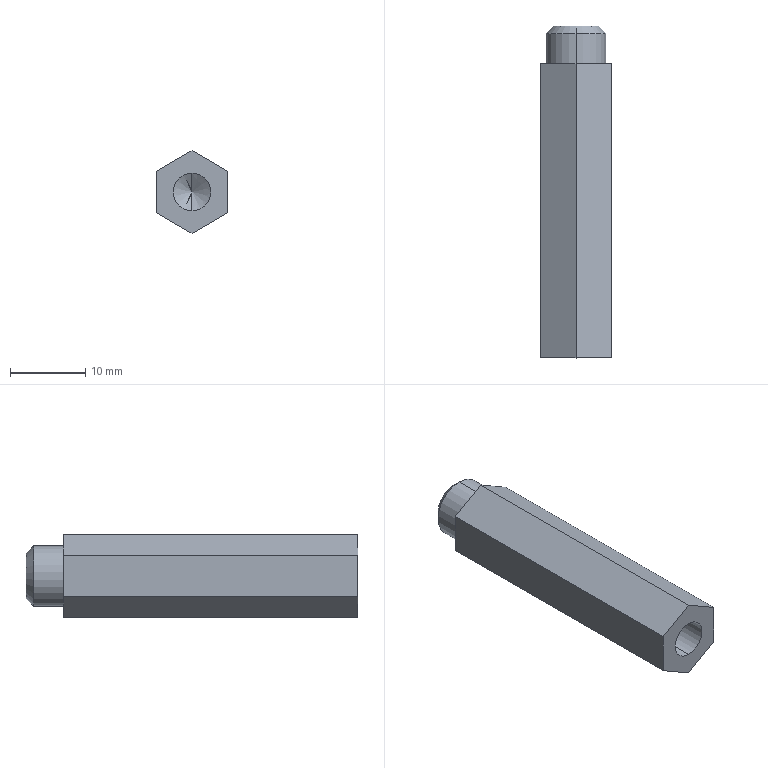Part | SolidWorks | features 3DProfileFeature 1, Chamfer 1, Extrusion 1, HoleWzd 1, ICE 1 | 1 solid | 17 faces | box 9.526 x 44 x 11 mm | volume 3138 mm3 | plane 9 | cylinder 4 | cone 4 | commonest cylinder face diameters 5 x2 8 x2
STEP:
#1=CARTESIAN_POINT('',(-0.000004548,-11.5,2.5));
#2=VERTEX_POINT('',#1);
#3=CARTESIAN_POINT('',(-0.000004548,-11.5,-2.5));
#4=VERTEX_POINT('',#3);
#5=CARTESIAN_POINT('',(-0.000004548,-11.5,0.00002582));
#6=DIRECTION('',(0.,-1.,0.));
#7=DIRECTION('',(0.,0.,-1.));
#8=AXIS2_PLACEMENT_3D('',#5,#6,#7);
#9=CIRCLE('',#8,2.5);
#10=EDGE_CURVE('',#2,#4,#9,.T.);
#11=ORIENTED_EDGE('',*,*,#10,.F.);
#12=CARTESIAN_POINT('',(-0.000004548,-19.5,2.5));
#13=VERTEX_POINT('',#12);
#14=CARTESIAN_POINT('',(-0.000004548,-19.5,2.5));
#15=DIRECTION('',(0.,-1.,0.));
#16=VECTOR('',#15,1000.);
#17=LINE('',#14,#16);
#18=EDGE_CURVE('',#2,#13,#17,.T.);
#19=ORIENTED_EDGE('',*,*,#18,.T.);
#20=CARTESIAN_POINT('',(-0.000004548,-19.5,-2.5));
#21=VERTEX_POINT('',#20);
#22=CARTESIAN_POINT('',(-0.000004548,-19.5,0.00002582));
#23=DIRECTION('',(0.,-1.,0.));
#24=DIRECTION('',(0.,0.,-1.));
#25=AXIS2_PLACEMENT_3D('',#22,#23,#24);
#26=CIRCLE('',#25,2.5);
#27=EDGE_CURVE('',#13,#21,#26,.T.);
#28=ORIENTED_EDGE('',*,*,#27,.T.);
#29=CARTESIAN_POINT('',(-0.000004548,-19.5,-2.5));
#30=DIRECTION('',(0.,-1.,0.));
#31=VECTOR('',#30,1000.);
#32=LINE('',#29,#31);
#33=EDGE_CURVE('',#4,#21,#32,.T.);
#34=ORIENTED_EDGE('',*,*,#33,.F.);
#35=EDGE_LOOP('',(#11,#19,#28,#34));
#36=FACE_OUTER_BOUND('',#35,.T.);
#37=CARTESIAN_POINT('',(-0.000004548,-19.5,0.00002582));
#38=DIRECTION('',(0.,-1.,0.));
#39=DIRECTION('',(0.,0.,-1.));
#40=AXIS2_PLACEMENT_3D('',#37,#38,#39);
#41=CYLINDRICAL_SURFACE('',#40,2.5);
#42=ADVANCED_FACE('',(#36),#41,.F.);
#43=CARTESIAN_POINT('',(-0.000004548,-9.998,0.00002582));
#44=VERTEX_POINT('',#43);
#45=CARTESIAN_POINT('',(-0.000004548,-11.5,-2.5));
#46=DIRECTION('',(0.,-0.515,-0.8572));
#47=VECTOR('',#46,1000.);
#48=LINE('',#45,#47);
#49=EDGE_CURVE('',#44,#4,#48,.T.);
#50=ORIENTED_EDGE('',*,*,#49,.F.);
#51=CARTESIAN_POINT('',(-0.000004548,-11.5,2.5));
#52=DIRECTION('',(0.,-0.515,0.8572));
#53=VECTOR('',#52,1000.);
#54=LINE('',#51,#53);
#55=EDGE_CURVE('',#44,#2,#54,.T.);
#56=ORIENTED_EDGE('',*,*,#55,.T.);
#57=ORIENTED_EDGE('',*,*,#10,.T.);
#58=EDGE_LOOP('',(#50,#56,#57));
#59=FACE_OUTER_BOUND('',#58,.T.);
#60=CARTESIAN_POINT('',(-0.000004548,-11.5,0.00002582));
#61=DIRECTION('',(0.,-1.,0.));
#62=DIRECTION('',(0.,0.,-1.));
#63=AXIS2_PLACEMENT_3D('',#60,#61,#62);
#64=CONICAL_SURFACE('',#63,2.5,1.03);
#65=ADVANCED_FACE('',(#59),#64,.F.);
#66=CARTESIAN_POINT('',(0.,24.5,3.));
#67=VERTEX_POINT('',#66);
#68=CARTESIAN_POINT('',(0.,24.5,-3.));
#69=VERTEX_POINT('',#68);
#70=CARTESIAN_POINT('',(0.,24.5,0.));
#71=DIRECTION('',(0.,1.,0.));
#72=DIRECTION('',(0.,0.,1.));
#73=AXIS2_PLACEMENT_3D('',#70,#71,#72);
#74=CIRCLE('',#73,3.);
#75=EDGE_CURVE('',#67,#69,#74,.T.);
#76=ORIENTED_EDGE('',*,*,#75,.F.);
#77=CARTESIAN_POINT('',(0.,23.5,4.));
#78=VERTEX_POINT('',#77);
#79=CARTESIAN_POINT('',(0.,24.5,3.));
#80=DIRECTION('',(0.,-0.7071,0.7071));
#81=VECTOR('',#80,1000.);
#82=LINE('',#79,#81);
#83=EDGE_CURVE('',#67,#78,#82,.T.);
#84=ORIENTED_EDGE('',*,*,#83,.T.);
#85=CARTESIAN_POINT('',(0.,23.5,-4.));
#86=VERTEX_POINT('',#85);
#87=CARTESIAN_POINT('',(0.,23.5,0.));
#88=DIRECTION('',(0.,-1.,0.));
#89=DIRECTION('',(0.,0.,1.));
#90=AXIS2_PLACEMENT_3D('',#87,#88,#89);
#91=CIRCLE('',#90,4.);
#92=EDGE_CURVE('',#86,#78,#91,.T.);
#93=ORIENTED_EDGE('',*,*,#92,.F.);
#94=CARTESIAN_POINT('',(0.,24.5,-3.));
#95=DIRECTION('',(0.,-0.7071,-0.7071));
#96=VECTOR('',#95,1000.);
#97=LINE('',#94,#96);
#98=EDGE_CURVE('',#69,#86,#97,.T.);
#99=ORIENTED_EDGE('',*,*,#98,.F.);
#100=EDGE_LOOP('',(#76,#84,#93,#99));
#101=FACE_OUTER_BOUND('',#100,.T.);
#102=CARTESIAN_POINT('',(0.,24.5,0.));
#103=DIRECTION('',(0.,-1.,0.));
#104=DIRECTION('',(0.,0.,-1.));
#105=AXIS2_PLACEMENT_3D('',#102,#103,#104);
#106=CONICAL_SURFACE('',#105,3.,0.7854);
#107=ADVANCED_FACE('',(#101),#106,.T.);
#108=ORIENTED_EDGE('',*,*,#92,.T.);
#109=CARTESIAN_POINT('',(0.,19.5,4.));
#110=VERTEX_POINT('',#109);
#111=CARTESIAN_POINT('',(0.,24.5,4.));
#112=DIRECTION('',(0.,-1.,0.));
#113=VECTOR('',#112,1000.);
#114=LINE('',#111,#113);
#115=EDGE_CURVE('',#78,#110,#114,.T.);
#116=ORIENTED_EDGE('',*,*,#115,.T.);
#117=CARTESIAN_POINT('',(0.,19.5,-4.));
#118=VERTEX_POINT('',#117);
#119=CARTESIAN_POINT('',(0.,19.5,0.));
#120=DIRECTION('',(0.,1.,0.));
#121=DIRECTION('',(0.,0.,1.));
#122=AXIS2_PLACEMENT_3D('',#119,#120,#121);
#123=CIRCLE('',#122,4.);
#124=EDGE_CURVE('',#110,#118,#123,.T.);
#125=ORIENTED_EDGE('',*,*,#124,.T.);
#126=CARTESIAN_POINT('',(0.,24.5,-4.));
#127=DIRECTION('',(0.,-1.,0.));
#128=VECTOR('',#127,1000.);
#129=LINE('',#126,#128);
#130=EDGE_CURVE('',#86,#118,#129,.T.);
#131=ORIENTED_EDGE('',*,*,#130,.F.);
#132=EDGE_LOOP('',(#108,#116,#125,#131));
#133=FACE_OUTER_BOUND('',#132,.T.);
#134=CARTESIAN_POINT('',(0.,24.5,0.));
#135=DIRECTION('',(0.,-1.,0.));
#136=DIRECTION('',(0.,0.,-1.));
#137=AXIS2_PLACEMENT_3D('',#134,#135,#136);
#138=CYLINDRICAL_SURFACE('',#137,4.);
#139=ADVANCED_FACE('',(#133),#138,.T.);
#140=CARTESIAN_POINT('',(4.763,19.5,-2.75));
#141=VERTEX_POINT('',#140);
#142=CARTESIAN_POINT('',(0.,19.5,-5.5));
#143=VERTEX_POINT('',#142);
#144=CARTESIAN_POINT('',(4.763,19.5,-2.75));
#145=DIRECTION('',(-0.866,0.,-0.5));
#146=VECTOR('',#145,1000.);
#147=LINE('',#144,#146);
#148=EDGE_CURVE('',#141,#143,#147,.T.);
#149=ORIENTED_EDGE('',*,*,#148,.T.);
#150=CARTESIAN_POINT('',(-4.763,19.5,-2.75));
#151=VERTEX_POINT('',#150);
#152=CARTESIAN_POINT('',(0.,19.5,-5.5));
#153=DIRECTION('',(-0.866,0.,0.5));
#154=VECTOR('',#153,1000.);
#155=LINE('',#152,#154);
#156=EDGE_CURVE('',#143,#151,#155,.T.);
#157=ORIENTED_EDGE('',*,*,#156,.T.);
#158=CARTESIAN_POINT('',(-4.763,19.5,2.75));
#159=VERTEX_POINT('',#158);
#160=CARTESIAN_POINT('',(-4.763,19.5,-2.75));
#161=DIRECTION('',(0.,0.,1.));
#162=VECTOR('',#161,1000.);
#163=LINE('',#160,#162);
#164=EDGE_CURVE('',#151,#159,#163,.T.);
#165=ORIENTED_EDGE('',*,*,#164,.T.);
#166=CARTESIAN_POINT('',(0.,19.5,5.5));
#167=VERTEX_POINT('',#166);
#168=CARTESIAN_POINT('',(-4.763,19.5,2.75));
#169=DIRECTION('',(0.866,0.,0.5));
#170=VECTOR('',#169,1000.);
#171=LINE('',#168,#170);
#172=EDGE_CURVE('',#159,#167,#171,.T.);
#173=ORIENTED_EDGE('',*,*,#172,.T.);
#174=CARTESIAN_POINT('',(4.763,19.5,2.75));
#175=VERTEX_POINT('',#174);
#176=CARTESIAN_POINT('',(0.,19.5,5.5));
#177=DIRECTION('',(0.866,0.,-0.5));
#178=VECTOR('',#177,1000.);
#179=LINE('',#176,#178);
#180=EDGE_CURVE('',#167,#175,#179,.T.);
#181=ORIENTED_EDGE('',*,*,#180,.T.);
#182=CARTESIAN_POINT('',(4.763,19.5,2.75));
#183=DIRECTION('',(0.,0.,-1.));
#184=VECTOR('',#183,1000.);
#185=LINE('',#182,#184);
#186=EDGE_CURVE('',#175,#141,#185,.T.);
#187=ORIENTED_EDGE('',*,*,#186,.T.);
#188=EDGE_LOOP('',(#149,#157,#165,#173,#181,#187));
#189=FACE_OUTER_BOUND('',#188,.T.);
#190=CARTESIAN_POINT('',(0.,19.5,0.));
#191=DIRECTION('',(0.,1.,0.));
#192=DIRECTION('',(0.,0.,1.));
#193=AXIS2_PLACEMENT_3D('',#190,#191,#192);
#194=CIRCLE('',#193,4.);
#195=EDGE_CURVE('',#118,#110,#194,.T.);
#196=ORIENTED_EDGE('',*,*,#195,.F.);
#197=ORIENTED_EDGE('',*,*,#124,.F.);
#198=EDGE_LOOP('',(#196,#197));
#199=FACE_BOUND('',#198,.T.);
#200=CARTESIAN_POINT('',(0.,19.5,0.));
#201=DIRECTION('',(0.,1.,0.));
#202=DIRECTION('',(0.,0.,1.));
#203=AXIS2_PLACEMENT_3D('',#200,#201,#202);
#204=PLANE('',#203);
#205=ADVANCED_FACE('',(#189,#199),#204,.T.);
#206=CARTESIAN_POINT('',(4.763,-19.5,-2.75));
#207=VERTEX_POINT('',#206);
#208=CARTESIAN_POINT('',(0.,-19.5,-5.5));
#209=VERTEX_POINT('',#208);
#210=CARTESIAN_POINT('',(4.763,-19.5,-2.75));
#211=DIRECTION('',(-0.866,0.,-0.5));
#212=VECTOR('',#211,1000.);
#213=LINE('',#210,#212);
#214=EDGE_CURVE('',#207,#209,#213,.T.);
#215=ORIENTED_EDGE('',*,*,#214,.T.);
#216=CARTESIAN_POINT('',(0.,19.5,-5.5));
#217=DIRECTION('',(0.,-1.,0.));
#218=VECTOR('',#217,1000.);
#219=LINE('',#216,#218);
#220=EDGE_CURVE('',#143,#209,#219,.T.);
#221=ORIENTED_EDGE('',*,*,#220,.F.);
#222=ORIENTED_EDGE('',*,*,#148,.F.);
#223=CARTESIAN_POINT('',(4.763,19.5,-2.75));
#224=DIRECTION('',(0.,-1.,0.));
#225=VECTOR('',#224,1000.);
#226=LINE('',#223,#225);
#227=EDGE_CURVE('',#141,#207,#226,.T.);
#228=ORIENTED_EDGE('',*,*,#227,.T.);
#229=EDGE_LOOP('',(#215,#221,#222,#228));
#230=FACE_OUTER_BOUND('',#229,.T.);
#231=CARTESIAN_POINT('',(4.763,19.5,-2.75));
#232=DIRECTION('',(-0.5,0.,0.866));
#233=DIRECTION('',(0.866,0.,0.5));
#234=AXIS2_PLACEMENT_3D('',#231,#232,#233);
#235=PLANE('',#234);
#236=ADVANCED_FACE('',(#230),#235,.F.);
#237=CARTESIAN_POINT('',(-4.763,-19.5,-2.75));
#238=VERTEX_POINT('',#237);
#239=CARTESIAN_POINT('',(0.,-19.5,-5.5));
#240=DIRECTION('',(-0.866,0.,0.5));
#241=VECTOR('',#240,1000.);
#242=LINE('',#239,#241);
#243=EDGE_CURVE('',#209,#238,#242,.T.);
#244=ORIENTED_EDGE('',*,*,#243,.T.);
#245=CARTESIAN_POINT('',(-4.763,19.5,-2.75));
#246=DIRECTION('',(0.,-1.,0.));
#247=VECTOR('',#246,1000.);
#248=LINE('',#245,#247);
#249=EDGE_CURVE('',#151,#238,#248,.T.);
#250=ORIENTED_EDGE('',*,*,#249,.F.);
#251=ORIENTED_EDGE('',*,*,#156,.F.);
#252=ORIENTED_EDGE('',*,*,#220,.T.);
#253=EDGE_LOOP('',(#244,#250,#251,#252));
#254=FACE_OUTER_BOUND('',#253,.T.);
#255=CARTESIAN_POINT('',(0.,19.5,-5.5));
#256=DIRECTION('',(0.5,0.,0.866));
#257=DIRECTION('',(0.866,0.,-0.5));
#258=AXIS2_PLACEMENT_3D('',#255,#256,#257);
#259=PLANE('',#258);
#260=ADVANCED_FACE('',(#254),#259,.F.);
#261=CARTESIAN_POINT('',(-4.763,-19.5,2.75));
#262=VERTEX_POINT('',#261);
#263=CARTESIAN_POINT('',(-4.763,-19.5,-2.75));
#264=DIRECTION('',(0.,0.,1.));
#265=VECTOR('',#264,1000.);
#266=LINE('',#263,#265);
#267=EDGE_CURVE('',#238,#262,#266,.T.);
#268=ORIENTED_EDGE('',*,*,#267,.T.);
#269=CARTESIAN_POINT('',(-4.763,19.5,2.75));
#270=DIRECTION('',(0.,-1.,0.));
#271=VECTOR('',#270,1000.);
#272=LINE('',#269,#271);
#273=EDGE_CURVE('',#159,#262,#272,.T.);
#274=ORIENTED_EDGE('',*,*,#273,.F.);
#275=ORIENTED_EDGE('',*,*,#164,.F.);
#276=ORIENTED_EDGE('',*,*,#249,.T.);
#277=EDGE_LOOP('',(#268,#274,#275,#276));
#278=FACE_OUTER_BOUND('',#277,.T.);
#279=CARTESIAN_POINT('',(-4.763,19.5,-2.75));
#280=DIRECTION('',(1.,0.,0.));
#281=DIRECTION('',(0.,0.,-1.));
#282=AXIS2_PLACEMENT_3D('',#279,#280,#281);
#283=PLANE('',#282);
#284=ADVANCED_FACE('',(#278),#283,.F.);
#285=CARTESIAN_POINT('',(0.,-19.5,5.5));
#286=VERTEX_POINT('',#285);
#287=CARTESIAN_POINT('',(-4.763,-19.5,2.75));
#288=DIRECTION('',(0.866,0.,0.5));
#289=VECTOR('',#288,1000.);
#290=LINE('',#287,#289);
#291=EDGE_CURVE('',#262,#286,#290,.T.);
#292=ORIENTED_EDGE('',*,*,#291,.T.);
#293=CARTESIAN_POINT('',(0.,19.5,5.5));
#294=DIRECTION('',(0.,-1.,0.));
#295=VECTOR('',#294,1000.);
#296=LINE('',#293,#295);
#297=EDGE_CURVE('',#167,#286,#296,.T.);
#298=ORIENTED_EDGE('',*,*,#297,.F.);
#299=ORIENTED_EDGE('',*,*,#172,.F.);
#300=ORIENTED_EDGE('',*,*,#273,.T.);
#301=EDGE_LOOP('',(#292,#298,#299,#300));
#302=FACE_OUTER_BOUND('',#301,.T.);
#303=CARTESIAN_POINT('',(-4.763,19.5,2.75));
#304=DIRECTION('',(0.5,0.,-0.866));
#305=DIRECTION('',(-0.866,0.,-0.5));
#306=AXIS2_PLACEMENT_3D('',#303,#304,#305);
#307=PLANE('',#306);
#308=ADVANCED_FACE('',(#302),#307,.F.);
#309=CARTESIAN_POINT('',(4.763,-19.5,2.75));
#310=VERTEX_POINT('',#309);
#311=CARTESIAN_POINT('',(0.,-19.5,5.5));
#312=DIRECTION('',(0.866,0.,-0.5));
#313=VECTOR('',#312,1000.);
#314=LINE('',#311,#313);
#315=EDGE_CURVE('',#286,#310,#314,.T.);
#316=ORIENTED_EDGE('',*,*,#315,.T.);
#317=CARTESIAN_POINT('',(4.763,19.5,2.75));
#318=DIRECTION('',(0.,-1.,0.));
#319=VECTOR('',#318,1000.);
#320=LINE('',#317,#319);
#321=EDGE_CURVE('',#175,#310,#320,.T.);
#322=ORIENTED_EDGE('',*,*,#321,.F.);
#323=ORIENTED_EDGE('',*,*,#180,.F.);
#324=ORIENTED_EDGE('',*,*,#297,.T.);
#325=EDGE_LOOP('',(#316,#322,#323,#324));
#326=FACE_OUTER_BOUND('',#325,.T.);
#327=CARTESIAN_POINT('',(0.,19.5,5.5));
#328=DIRECTION('',(-0.5,0.,-0.866));
#329=DIRECTION('',(-0.866,0.,0.5));
#330=AXIS2_PLACEMENT_3D('',#327,#328,#329);
#331=PLANE('',#330);
#332=ADVANCED_FACE('',(#326),#331,.F.);
#333=CARTESIAN_POINT('',(4.763,-19.5,2.75));
#334=DIRECTION('',(0.,0.,-1.));
#335=VECTOR('',#334,1000.);
#336=LINE('',#333,#335);
#337=EDGE_CURVE('',#310,#207,#336,.T.);
#338=ORIENTED_EDGE('',*,*,#337,.T.);
#339=ORIENTED_EDGE('',*,*,#227,.F.);
#340=ORIENTED_EDGE('',*,*,#186,.F.);
#341=ORIENTED_EDGE('',*,*,#321,.T.);
#342=EDGE_LOOP('',(#338,#339,#340,#341));
#343=FACE_OUTER_BOUND('',#342,.T.);
#344=CARTESIAN_POINT('',(4.763,19.5,2.75));
#345=DIRECTION('',(-1.,0.,0.));
#346=DIRECTION('',(0.,0.,1.));
#347=AXIS2_PLACEMENT_3D('',#344,#345,#346);
#348=PLANE('',#347);
#349=ADVANCED_FACE('',(#343),#348,.F.);
#350=CARTESIAN_POINT('',(-0.000004548,-19.5,0.00002582));
#351=DIRECTION('',(0.,-1.,0.));
#352=DIRECTION('',(0.,0.,-1.));
#353=AXIS2_PLACEMENT_3D('',#350,#351,#352);
#354=CIRCLE('',#353,2.5);
#355=EDGE_CURVE('',#21,#13,#354,.T.);
#356=ORIENTED_EDGE('',*,*,#355,.F.);
#357=ORIENTED_EDGE('',*,*,#27,.F.);
#358=EDGE_LOOP('',(#356,#357));
#359=FACE_BOUND('',#358,.T.);
#360=ORIENTED_EDGE('',*,*,#214,.F.);
#361=ORIENTED_EDGE('',*,*,#337,.F.);
#362=ORIENTED_EDGE('',*,*,#315,.F.);
#363=ORIENTED_EDGE('',*,*,#291,.F.);
#364=ORIENTED_EDGE('',*,*,#267,.F.);
#365=ORIENTED_EDGE('',*,*,#243,.F.);
#366=EDGE_LOOP('',(#360,#361,#362,#363,#364,#365));
#367=FACE_OUTER_BOUND('',#366,.T.);
#368=CARTESIAN_POINT('',(0.,-19.5,0.));
#369=DIRECTION('',(0.,1.,0.));
#370=DIRECTION('',(0.,0.,1.));
#371=AXIS2_PLACEMENT_3D('',#368,#369,#370);
#372=PLANE('',#371);
#373=ADVANCED_FACE('',(#359,#367),#372,.F.);
#374=ORIENTED_EDGE('',*,*,#115,.F.);
#375=CARTESIAN_POINT('',(0.,23.5,0.));
#376=DIRECTION('',(0.,-1.,0.));
#377=DIRECTION('',(0.,0.,1.));
#378=AXIS2_PLACEMENT_3D('',#375,#376,#377);
#379=CIRCLE('',#378,4.);
#380=EDGE_CURVE('',#78,#86,#379,.T.);
#381=ORIENTED_EDGE('',*,*,#380,.T.);
#382=ORIENTED_EDGE('',*,*,#130,.T.);
#383=ORIENTED_EDGE('',*,*,#195,.T.);
#384=EDGE_LOOP('',(#374,#381,#382,#383));
#385=FACE_OUTER_BOUND('',#384,.T.);
#386=CARTESIAN_POINT('',(0.,24.5,0.));
#387=DIRECTION('',(0.,-1.,0.));
#388=DIRECTION('',(0.,0.,-1.));
#389=AXIS2_PLACEMENT_3D('',#386,#387,#388);
#390=CYLINDRICAL_SURFACE('',#389,4.);
#391=ADVANCED_FACE('',(#385),#390,.T.);
#392=CARTESIAN_POINT('',(0.,24.5,0.));
#393=DIRECTION('',(0.,1.,0.));
#394=DIRECTION('',(0.,0.,1.));
#395=AXIS2_PLACEMENT_3D('',#392,#393,#394);
#396=CIRCLE('',#395,3.);
#397=EDGE_CURVE('',#69,#67,#396,.T.);
#398=ORIENTED_EDGE('',*,*,#397,.T.);
#399=ORIENTED_EDGE('',*,*,#75,.T.);
#400=EDGE_LOOP('',(#398,#399));
#401=FACE_OUTER_BOUND('',#400,.T.);
#402=CARTESIAN_POINT('',(0.,24.5,0.));
#403=DIRECTION('',(0.,1.,0.));
#404=DIRECTION('',(0.,0.,1.));
#405=AXIS2_PLACEMENT_3D('',#402,#403,#404);
#406=PLANE('',#405);
#407=ADVANCED_FACE('',(#401),#406,.T.);
#408=ORIENTED_EDGE('',*,*,#83,.F.);
#409=ORIENTED_EDGE('',*,*,#397,.F.);
#410=ORIENTED_EDGE('',*,*,#98,.T.);
#411=ORIENTED_EDGE('',*,*,#380,.F.);
#412=EDGE_LOOP('',(#408,#409,#410,#411));
#413=FACE_OUTER_BOUND('',#412,.T.);
#414=CARTESIAN_POINT('',(0.,24.5,0.));
#415=DIRECTION('',(0.,-1.,0.));
#416=DIRECTION('',(0.,0.,-1.));
#417=AXIS2_PLACEMENT_3D('',#414,#415,#416);
#418=CONICAL_SURFACE('',#417,3.,0.7854);
#419=ADVANCED_FACE('',(#413),#418,.T.);
#420=ORIENTED_EDGE('',*,*,#55,.F.);
#421=ORIENTED_EDGE('',*,*,#49,.T.);
#422=CARTESIAN_POINT('',(-0.000004548,-11.5,0.00002582));
#423=DIRECTION('',(0.,-1.,0.));
#424=DIRECTION('',(0.,0.,-1.));
#425=AXIS2_PLACEMENT_3D('',#422,#423,#424);
#426=CIRCLE('',#425,2.5);
#427=EDGE_CURVE('',#4,#2,#426,.T.);
#428=ORIENTED_EDGE('',*,*,#427,.T.);
#429=EDGE_LOOP('',(#420,#421,#428));
#430=FACE_OUTER_BOUND('',#429,.T.);
#431=CARTESIAN_POINT('',(-0.000004548,-11.5,0.00002582));
#432=DIRECTION('',(0.,-1.,0.));
#433=DIRECTION('',(0.,0.,-1.));
#434=AXIS2_PLACEMENT_3D('',#431,#432,#433);
#435=CONICAL_SURFACE('',#434,2.5,1.03);
#436=ADVANCED_FACE('',(#430),#435,.F.);
#437=ORIENTED_EDGE('',*,*,#18,.F.);
#438=ORIENTED_EDGE('',*,*,#427,.F.);
#439=ORIENTED_EDGE('',*,*,#33,.T.);
#440=ORIENTED_EDGE('',*,*,#355,.T.);
#441=EDGE_LOOP('',(#437,#438,#439,#440));
#442=FACE_OUTER_BOUND('',#441,.T.);
#443=CARTESIAN_POINT('',(-0.000004548,-19.5,0.00002582));
#444=DIRECTION('',(0.,-1.,0.));
#445=DIRECTION('',(0.,0.,-1.));
#446=AXIS2_PLACEMENT_3D('',#443,#444,#445);
#447=CYLINDRICAL_SURFACE('',#446,2.5);
#448=ADVANCED_FACE('',(#442),#447,.F.);
#449=CLOSED_SHELL('',(#42,#65,#107,#139,#205,#236,#260,#284,#308,#332,#349,#373,#391,#407,#419,#436,#448));
#450=MANIFOLD_SOLID_BREP('',#449);
#451=CARTESIAN_POINT('',(0.,0.,0.));
#452=DIRECTION('',(0.,0.,1.));
#453=DIRECTION('',(1.,0.,0.));
#454=AXIS2_PLACEMENT_3D('',#451,#452,#453);
#455=(LENGTH_UNIT()NAMED_UNIT(*)SI_UNIT(.MILLI.,.METRE.));
#456=UNCERTAINTY_MEASURE_WITH_UNIT(LENGTH_MEASURE(0.00001),#455,'','');
#457=(NAMED_UNIT(*)PLANE_ANGLE_UNIT()SI_UNIT($,.RADIAN.));
#458=(NAMED_UNIT(*)SI_UNIT($,.STERADIAN.)SOLID_ANGLE_UNIT());
#459=(GEOMETRIC_REPRESENTATION_CONTEXT(3)GLOBAL_UNCERTAINTY_ASSIGNED_CONTEXT((#456))GLOBAL_UNIT_ASSIGNED_CONTEXT((#455,#457,#458))REPRESENTATION_CONTEXT('',''));
#460=ADVANCED_BREP_SHAPE_REPRESENTATION('',(#450,#454),#459);